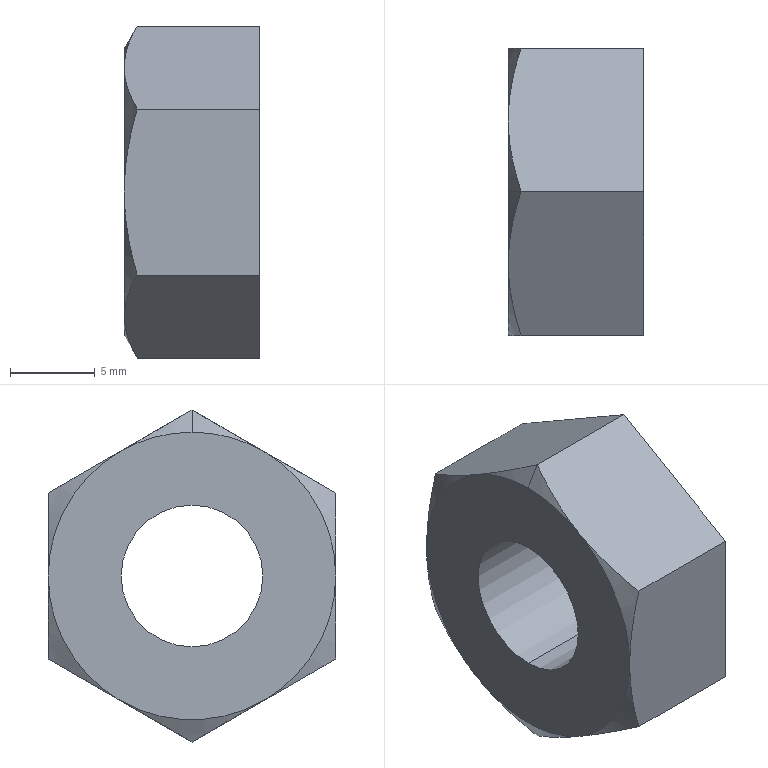Part | STEP file | Eyebolt mounting bracket-Part-4 | 1 solid | 17 faces | box 8 x 17 x 19.63 mm | volume 1556 mm3 | plane 8 | cone 7 | cylinder 2 | commonest cylinder face diameters 8.376 x2